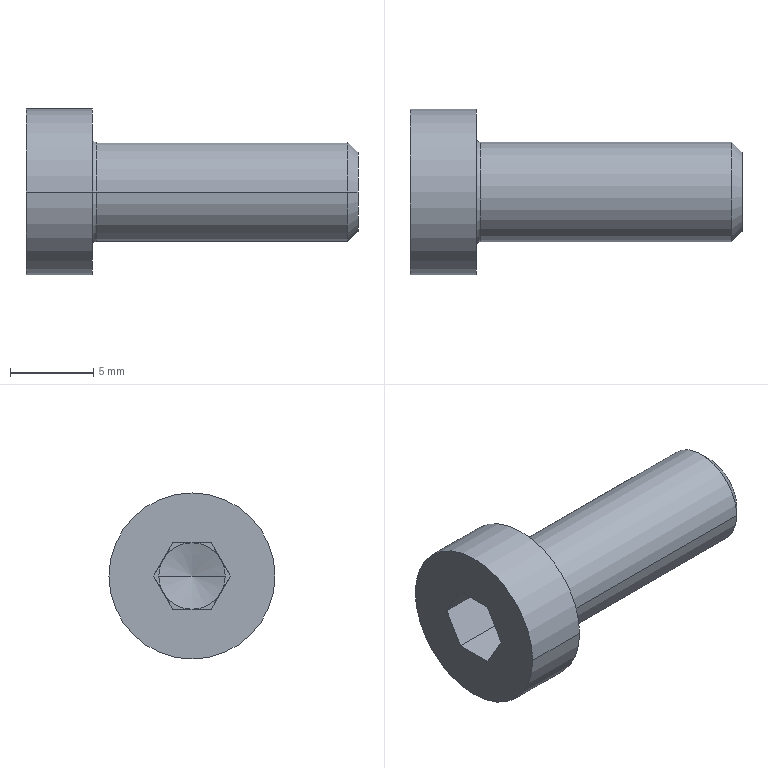Part | STEP file | CBSSTH6-16 | 1 solid | 25 faces | box 20 x 10 x 10 mm | volume 719.687 mm3 | plane 15 | cone 4 | cylinder 4 | torus 2 | commonest cylinder face diameters 6 x2 10 x2
STEP:
#1=CARTESIAN_POINT('',(-0.4641,0.,0.));
#2=VERTEX_POINT('',#1);
#3=CARTESIAN_POINT('',(-1.,-2.,0.));
#4=VERTEX_POINT('',#3);
#5=CARTESIAN_POINT('',(-0.4641,0.,0.));
#6=DIRECTION('',(-0.2588,-0.9659,0.));
#7=VECTOR('',#6,1000.);
#8=LINE('',#5,#7);
#9=EDGE_CURVE('',#2,#4,#8,.T.);
#10=ORIENTED_EDGE('',*,*,#9,.F.);
#11=CARTESIAN_POINT('',(-1.,2.,0.));
#12=VERTEX_POINT('',#11);
#13=CARTESIAN_POINT('',(-0.4641,0.,0.));
#14=DIRECTION('',(-0.2588,0.9659,0.));
#15=VECTOR('',#14,1000.);
#16=LINE('',#13,#15);
#17=EDGE_CURVE('',#2,#12,#16,.T.);
#18=ORIENTED_EDGE('',*,*,#17,.T.);
#19=CARTESIAN_POINT('',(-1.,1.732,-1.));
#20=VERTEX_POINT('',#19);
#21=CARTESIAN_POINT('',(-1.,0.,0.));
#22=DIRECTION('',(1.,0.,0.));
#23=DIRECTION('',(0.,1.,0.));
#24=AXIS2_PLACEMENT_3D('',#21,#22,#23);
#25=CIRCLE('',#24,2.);
#26=EDGE_CURVE('',#20,#12,#25,.T.);
#27=ORIENTED_EDGE('',*,*,#26,.F.);
#28=CARTESIAN_POINT('',(-1.,0.,-2.));
#29=VERTEX_POINT('',#28);
#30=CARTESIAN_POINT('',(-1.,0.,0.));
#31=DIRECTION('',(1.,0.,0.));
#32=DIRECTION('',(0.,1.,0.));
#33=AXIS2_PLACEMENT_3D('',#30,#31,#32);
#34=CIRCLE('',#33,2.);
#35=EDGE_CURVE('',#29,#20,#34,.T.);
#36=ORIENTED_EDGE('',*,*,#35,.F.);
#37=CARTESIAN_POINT('',(-1.,-1.732,-1.));
#38=VERTEX_POINT('',#37);
#39=CARTESIAN_POINT('',(-1.,0.,0.));
#40=DIRECTION('',(1.,0.,0.));
#41=DIRECTION('',(0.,1.,0.));
#42=AXIS2_PLACEMENT_3D('',#39,#40,#41);
#43=CIRCLE('',#42,2.);
#44=EDGE_CURVE('',#38,#29,#43,.T.);
#45=ORIENTED_EDGE('',*,*,#44,.F.);
#46=CARTESIAN_POINT('',(-1.,0.,0.));
#47=DIRECTION('',(1.,0.,0.));
#48=DIRECTION('',(0.,1.,0.));
#49=AXIS2_PLACEMENT_3D('',#46,#47,#48);
#50=CIRCLE('',#49,2.);
#51=EDGE_CURVE('',#4,#38,#50,.T.);
#52=ORIENTED_EDGE('',*,*,#51,.F.);
#53=EDGE_LOOP('',(#10,#18,#27,#36,#45,#52));
#54=FACE_OUTER_BOUND('',#53,.T.);
#55=CARTESIAN_POINT('',(-1000.464,0.,0.));
#56=DIRECTION('',(-1.,0.,0.));
#57=DIRECTION('',(0.,-1.,0.));
#58=AXIS2_PLACEMENT_3D('',#55,#56,#57);
#59=CONICAL_SURFACE('',#58,3732.051,1.309);
#60=ADVANCED_FACE('',(#54),#59,.F.);
#61=CARTESIAN_POINT('',(16.,2.387,0.));
#62=VERTEX_POINT('',#61);
#63=CARTESIAN_POINT('',(16.,-2.387,0.));
#64=VERTEX_POINT('',#63);
#65=CARTESIAN_POINT('',(16.,0.,0.));
#66=DIRECTION('',(1.,0.,0.));
#67=DIRECTION('',(0.,1.,0.));
#68=AXIS2_PLACEMENT_3D('',#65,#66,#67);
#69=CIRCLE('',#68,2.387);
#70=EDGE_CURVE('',#62,#64,#69,.T.);
#71=ORIENTED_EDGE('',*,*,#70,.F.);
#72=CARTESIAN_POINT('',(15.386,3.,0.));
#73=VERTEX_POINT('',#72);
#74=CARTESIAN_POINT('',(15.386,3.,0.));
#75=DIRECTION('',(-0.7071,0.7071,0.));
#76=VECTOR('',#75,1000.);
#77=LINE('',#74,#76);
#78=EDGE_CURVE('',#62,#73,#77,.T.);
#79=ORIENTED_EDGE('',*,*,#78,.T.);
#80=CARTESIAN_POINT('',(15.386,-3.,0.));
#81=VERTEX_POINT('',#80);
#82=CARTESIAN_POINT('',(15.386,0.,0.));
#83=DIRECTION('',(1.,0.,0.));
#84=DIRECTION('',(0.,1.,0.));
#85=AXIS2_PLACEMENT_3D('',#82,#83,#84);
#86=CIRCLE('',#85,3.);
#87=EDGE_CURVE('',#73,#81,#86,.T.);
#88=ORIENTED_EDGE('',*,*,#87,.T.);
#89=CARTESIAN_POINT('',(15.386,-3.,0.));
#90=DIRECTION('',(-0.7071,-0.7071,0.));
#91=VECTOR('',#90,1000.);
#92=LINE('',#89,#91);
#93=EDGE_CURVE('',#64,#81,#92,.T.);
#94=ORIENTED_EDGE('',*,*,#93,.F.);
#95=EDGE_LOOP('',(#71,#79,#88,#94));
#96=FACE_OUTER_BOUND('',#95,.T.);
#97=CARTESIAN_POINT('',(15.386,0.,0.));
#98=DIRECTION('',(-1.,0.,0.));
#99=DIRECTION('',(0.,-1.,0.));
#100=AXIS2_PLACEMENT_3D('',#97,#98,#99);
#101=CONICAL_SURFACE('',#100,3.,0.7854);
#102=ADVANCED_FACE('',(#96),#101,.T.);
#103=CARTESIAN_POINT('',(0.25,3.,0.));
#104=VERTEX_POINT('',#103);
#105=CARTESIAN_POINT('',(0.25,-3.,0.));
#106=VERTEX_POINT('',#105);
#107=CARTESIAN_POINT('',(0.25,0.,0.));
#108=DIRECTION('',(1.,0.,0.));
#109=DIRECTION('',(0.,1.,0.));
#110=AXIS2_PLACEMENT_3D('',#107,#108,#109);
#111=CIRCLE('',#110,3.);
#112=EDGE_CURVE('',#104,#106,#111,.T.);
#113=ORIENTED_EDGE('',*,*,#112,.T.);
#114=CARTESIAN_POINT('',(16.,-3.,0.));
#115=DIRECTION('',(1.,0.,0.));
#116=VECTOR('',#115,1000.);
#117=LINE('',#114,#116);
#118=EDGE_CURVE('',#106,#81,#117,.T.);
#119=ORIENTED_EDGE('',*,*,#118,.T.);
#120=ORIENTED_EDGE('',*,*,#87,.F.);
#121=CARTESIAN_POINT('',(16.,3.,0.));
#122=DIRECTION('',(1.,0.,0.));
#123=VECTOR('',#122,1000.);
#124=LINE('',#121,#123);
#125=EDGE_CURVE('',#104,#73,#124,.T.);
#126=ORIENTED_EDGE('',*,*,#125,.F.);
#127=EDGE_LOOP('',(#113,#119,#120,#126));
#128=FACE_OUTER_BOUND('',#127,.T.);
#129=CARTESIAN_POINT('',(16.,0.,0.));
#130=DIRECTION('',(1.,0.,0.));
#131=DIRECTION('',(0.,1.,0.));
#132=AXIS2_PLACEMENT_3D('',#129,#130,#131);
#133=CYLINDRICAL_SURFACE('',#132,3.);
#134=ADVANCED_FACE('',(#128),#133,.T.);
#135=CARTESIAN_POINT('',(0.25,0.,0.));
#136=DIRECTION('',(1.,0.,0.));
#137=DIRECTION('',(0.,1.,0.));
#138=AXIS2_PLACEMENT_3D('',#135,#136,#137);
#139=CIRCLE('',#138,3.);
#140=EDGE_CURVE('',#106,#104,#139,.T.);
#141=ORIENTED_EDGE('',*,*,#140,.F.);
#142=CARTESIAN_POINT('',(0.,-3.25,0.));
#143=VERTEX_POINT('',#142);
#144=CARTESIAN_POINT('',(0.25,-3.25,0.));
#145=DIRECTION('',(0.,0.,1.));
#146=DIRECTION('',(0.,-1.,0.));
#147=AXIS2_PLACEMENT_3D('',#144,#145,#146);
#148=CIRCLE('',#147,0.25);
#149=EDGE_CURVE('',#106,#143,#148,.T.);
#150=ORIENTED_EDGE('',*,*,#149,.T.);
#151=CARTESIAN_POINT('',(0.,3.25,0.));
#152=VERTEX_POINT('',#151);
#153=CARTESIAN_POINT('',(0.,0.,0.));
#154=DIRECTION('',(1.,0.,0.));
#155=DIRECTION('',(0.,1.,0.));
#156=AXIS2_PLACEMENT_3D('',#153,#154,#155);
#157=CIRCLE('',#156,3.25);
#158=EDGE_CURVE('',#143,#152,#157,.T.);
#159=ORIENTED_EDGE('',*,*,#158,.T.);
#160=CARTESIAN_POINT('',(0.25,3.25,0.));
#161=DIRECTION('',(0.,0.,-1.));
#162=DIRECTION('',(-1.,0.,0.));
#163=AXIS2_PLACEMENT_3D('',#160,#161,#162);
#164=CIRCLE('',#163,0.25);
#165=EDGE_CURVE('',#104,#152,#164,.T.);
#166=ORIENTED_EDGE('',*,*,#165,.F.);
#167=EDGE_LOOP('',(#141,#150,#159,#166));
#168=FACE_OUTER_BOUND('',#167,.T.);
#169=CARTESIAN_POINT('',(0.25,0.,0.));
#170=DIRECTION('',(1.,0.,0.));
#171=DIRECTION('',(0.,1.,0.));
#172=AXIS2_PLACEMENT_3D('',#169,#170,#171);
#173=TOROIDAL_SURFACE('',#172,3.25,0.25);
#174=ADVANCED_FACE('',(#168),#173,.F.);
#175=CARTESIAN_POINT('',(-4.,5.,0.));
#176=VERTEX_POINT('',#175);
#177=CARTESIAN_POINT('',(-4.,-5.,0.));
#178=VERTEX_POINT('',#177);
#179=CARTESIAN_POINT('',(-4.,0.,0.));
#180=DIRECTION('',(1.,0.,0.));
#181=DIRECTION('',(0.,1.,0.));
#182=AXIS2_PLACEMENT_3D('',#179,#180,#181);
#183=CIRCLE('',#182,5.);
#184=EDGE_CURVE('',#176,#178,#183,.T.);
#185=ORIENTED_EDGE('',*,*,#184,.T.);
#186=CARTESIAN_POINT('',(0.,-5.,0.));
#187=VERTEX_POINT('',#186);
#188=CARTESIAN_POINT('',(16.,-5.,0.));
#189=DIRECTION('',(1.,0.,0.));
#190=VECTOR('',#189,1000.);
#191=LINE('',#188,#190);
#192=EDGE_CURVE('',#178,#187,#191,.T.);
#193=ORIENTED_EDGE('',*,*,#192,.T.);
#194=CARTESIAN_POINT('',(0.,5.,0.));
#195=VERTEX_POINT('',#194);
#196=CARTESIAN_POINT('',(0.,0.,0.));
#197=DIRECTION('',(1.,0.,0.));
#198=DIRECTION('',(0.,1.,0.));
#199=AXIS2_PLACEMENT_3D('',#196,#197,#198);
#200=CIRCLE('',#199,5.);
#201=EDGE_CURVE('',#195,#187,#200,.T.);
#202=ORIENTED_EDGE('',*,*,#201,.F.);
#203=CARTESIAN_POINT('',(16.,5.,0.));
#204=DIRECTION('',(1.,0.,0.));
#205=VECTOR('',#204,1000.);
#206=LINE('',#203,#205);
#207=EDGE_CURVE('',#176,#195,#206,.T.);
#208=ORIENTED_EDGE('',*,*,#207,.F.);
#209=EDGE_LOOP('',(#185,#193,#202,#208));
#210=FACE_OUTER_BOUND('',#209,.T.);
#211=CARTESIAN_POINT('',(16.,0.,0.));
#212=DIRECTION('',(1.,0.,0.));
#213=DIRECTION('',(0.,1.,0.));
#214=AXIS2_PLACEMENT_3D('',#211,#212,#213);
#215=CYLINDRICAL_SURFACE('',#214,5.);
#216=ADVANCED_FACE('',(#210),#215,.T.);
#217=ORIENTED_EDGE('',*,*,#184,.F.);
#218=CARTESIAN_POINT('',(-4.,0.,0.));
#219=DIRECTION('',(1.,0.,0.));
#220=DIRECTION('',(0.,1.,0.));
#221=AXIS2_PLACEMENT_3D('',#218,#219,#220);
#222=CIRCLE('',#221,5.);
#223=EDGE_CURVE('',#178,#176,#222,.T.);
#224=ORIENTED_EDGE('',*,*,#223,.F.);
#225=EDGE_LOOP('',(#217,#224));
#226=FACE_OUTER_BOUND('',#225,.T.);
#227=CARTESIAN_POINT('',(-4.,-1.155,-2.));
#228=VERTEX_POINT('',#227);
#229=CARTESIAN_POINT('',(-4.,-2.309,0.));
#230=VERTEX_POINT('',#229);
#231=CARTESIAN_POINT('',(-4.,-1.232,-1.866));
#232=DIRECTION('',(0.,-0.5,0.866));
#233=VECTOR('',#232,1000.);
#234=LINE('',#231,#233);
#235=EDGE_CURVE('',#228,#230,#234,.T.);
#236=ORIENTED_EDGE('',*,*,#235,.F.);
#237=CARTESIAN_POINT('',(-4.,1.155,-2.));
#238=VERTEX_POINT('',#237);
#239=CARTESIAN_POINT('',(-4.,2.,-2.));
#240=DIRECTION('',(0.,-1.,0.));
#241=VECTOR('',#240,1000.);
#242=LINE('',#239,#241);
#243=EDGE_CURVE('',#238,#228,#242,.T.);
#244=ORIENTED_EDGE('',*,*,#243,.F.);
#245=CARTESIAN_POINT('',(-4.,2.309,0.));
#246=VERTEX_POINT('',#245);
#247=CARTESIAN_POINT('',(-4.,2.232,-0.134));
#248=DIRECTION('',(0.,-0.5,-0.866));
#249=VECTOR('',#248,1000.);
#250=LINE('',#247,#249);
#251=EDGE_CURVE('',#246,#238,#250,.T.);
#252=ORIENTED_EDGE('',*,*,#251,.F.);
#253=CARTESIAN_POINT('',(-4.,1.155,2.));
#254=VERTEX_POINT('',#253);
#255=CARTESIAN_POINT('',(-4.,2.232,0.134));
#256=DIRECTION('',(0.,0.5,-0.866));
#257=VECTOR('',#256,1000.);
#258=LINE('',#255,#257);
#259=EDGE_CURVE('',#254,#246,#258,.T.);
#260=ORIENTED_EDGE('',*,*,#259,.F.);
#261=CARTESIAN_POINT('',(-4.,-1.155,2.));
#262=VERTEX_POINT('',#261);
#263=CARTESIAN_POINT('',(-4.,2.,2.));
#264=DIRECTION('',(0.,1.,0.));
#265=VECTOR('',#264,1000.);
#266=LINE('',#263,#265);
#267=EDGE_CURVE('',#262,#254,#266,.T.);
#268=ORIENTED_EDGE('',*,*,#267,.F.);
#269=CARTESIAN_POINT('',(-4.,-1.232,1.866));
#270=DIRECTION('',(0.,0.5,0.866));
#271=VECTOR('',#270,1000.);
#272=LINE('',#269,#271);
#273=EDGE_CURVE('',#230,#262,#272,.T.);
#274=ORIENTED_EDGE('',*,*,#273,.F.);
#275=EDGE_LOOP('',(#236,#244,#252,#260,#268,#274));
#276=FACE_BOUND('',#275,.T.);
#277=CARTESIAN_POINT('',(-4.,2.,0.));
#278=DIRECTION('',(1.,0.,0.));
#279=DIRECTION('',(0.,1.,0.));
#280=AXIS2_PLACEMENT_3D('',#277,#278,#279);
#281=PLANE('',#280);
#282=ADVANCED_FACE('',(#226,#276),#281,.F.);
#283=ORIENTED_EDGE('',*,*,#192,.F.);
#284=ORIENTED_EDGE('',*,*,#223,.T.);
#285=ORIENTED_EDGE('',*,*,#207,.T.);
#286=CARTESIAN_POINT('',(0.,0.,0.));
#287=DIRECTION('',(1.,0.,0.));
#288=DIRECTION('',(0.,1.,0.));
#289=AXIS2_PLACEMENT_3D('',#286,#287,#288);
#290=CIRCLE('',#289,5.);
#291=EDGE_CURVE('',#187,#195,#290,.T.);
#292=ORIENTED_EDGE('',*,*,#291,.F.);
#293=EDGE_LOOP('',(#283,#284,#285,#292));
#294=FACE_OUTER_BOUND('',#293,.T.);
#295=CARTESIAN_POINT('',(16.,0.,0.));
#296=DIRECTION('',(1.,0.,0.));
#297=DIRECTION('',(0.,1.,0.));
#298=AXIS2_PLACEMENT_3D('',#295,#296,#297);
#299=CYLINDRICAL_SURFACE('',#298,5.);
#300=ADVANCED_FACE('',(#294),#299,.T.);
#301=CARTESIAN_POINT('',(0.,0.,0.));
#302=DIRECTION('',(1.,0.,0.));
#303=DIRECTION('',(0.,1.,0.));
#304=AXIS2_PLACEMENT_3D('',#301,#302,#303);
#305=CIRCLE('',#304,3.25);
#306=EDGE_CURVE('',#152,#143,#305,.T.);
#307=ORIENTED_EDGE('',*,*,#306,.F.);
#308=ORIENTED_EDGE('',*,*,#158,.F.);
#309=EDGE_LOOP('',(#307,#308));
#310=FACE_BOUND('',#309,.T.);
#311=ORIENTED_EDGE('',*,*,#201,.T.);
#312=ORIENTED_EDGE('',*,*,#291,.T.);
#313=EDGE_LOOP('',(#311,#312));
#314=FACE_OUTER_BOUND('',#313,.T.);
#315=CARTESIAN_POINT('',(0.,5.,0.));
#316=DIRECTION('',(-1.,0.,0.));
#317=DIRECTION('',(0.,-1.,0.));
#318=AXIS2_PLACEMENT_3D('',#315,#316,#317);
#319=PLANE('',#318);
#320=ADVANCED_FACE('',(#310,#314),#319,.F.);
#321=ORIENTED_EDGE('',*,*,#149,.F.);
#322=ORIENTED_EDGE('',*,*,#112,.F.);
#323=ORIENTED_EDGE('',*,*,#165,.T.);
#324=ORIENTED_EDGE('',*,*,#306,.T.);
#325=EDGE_LOOP('',(#321,#322,#323,#324));
#326=FACE_OUTER_BOUND('',#325,.T.);
#327=CARTESIAN_POINT('',(0.25,0.,0.));
#328=DIRECTION('',(1.,0.,0.));
#329=DIRECTION('',(0.,1.,0.));
#330=AXIS2_PLACEMENT_3D('',#327,#328,#329);
#331=TOROIDAL_SURFACE('',#330,3.25,0.25);
#332=ADVANCED_FACE('',(#326),#331,.F.);
#333=ORIENTED_EDGE('',*,*,#118,.F.);
#334=ORIENTED_EDGE('',*,*,#140,.T.);
#335=ORIENTED_EDGE('',*,*,#125,.T.);
#336=CARTESIAN_POINT('',(15.386,0.,0.));
#337=DIRECTION('',(1.,0.,0.));
#338=DIRECTION('',(0.,1.,0.));
#339=AXIS2_PLACEMENT_3D('',#336,#337,#338);
#340=CIRCLE('',#339,3.);
#341=EDGE_CURVE('',#81,#73,#340,.T.);
#342=ORIENTED_EDGE('',*,*,#341,.F.);
#343=EDGE_LOOP('',(#333,#334,#335,#342));
#344=FACE_OUTER_BOUND('',#343,.T.);
#345=CARTESIAN_POINT('',(16.,0.,0.));
#346=DIRECTION('',(1.,0.,0.));
#347=DIRECTION('',(0.,1.,0.));
#348=AXIS2_PLACEMENT_3D('',#345,#346,#347);
#349=CYLINDRICAL_SURFACE('',#348,3.);
#350=ADVANCED_FACE('',(#344),#349,.T.);
#351=ORIENTED_EDGE('',*,*,#78,.F.);
#352=CARTESIAN_POINT('',(16.,0.,0.));
#353=DIRECTION('',(1.,0.,0.));
#354=DIRECTION('',(0.,1.,0.));
#355=AXIS2_PLACEMENT_3D('',#352,#353,#354);
#356=CIRCLE('',#355,2.387);
#357=EDGE_CURVE('',#64,#62,#356,.T.);
#358=ORIENTED_EDGE('',*,*,#357,.F.);
#359=ORIENTED_EDGE('',*,*,#93,.T.);
#360=ORIENTED_EDGE('',*,*,#341,.T.);
#361=EDGE_LOOP('',(#351,#358,#359,#360));
#362=FACE_OUTER_BOUND('',#361,.T.);
#363=CARTESIAN_POINT('',(15.386,0.,0.));
#364=DIRECTION('',(-1.,0.,0.));
#365=DIRECTION('',(0.,-1.,0.));
#366=AXIS2_PLACEMENT_3D('',#363,#364,#365);
#367=CONICAL_SURFACE('',#366,3.,0.7854);
#368=ADVANCED_FACE('',(#362),#367,.T.);
#369=ORIENTED_EDGE('',*,*,#357,.T.);
#370=ORIENTED_EDGE('',*,*,#70,.T.);
#371=EDGE_LOOP('',(#369,#370));
#372=FACE_OUTER_BOUND('',#371,.T.);
#373=CARTESIAN_POINT('',(16.,2.387,0.));
#374=DIRECTION('',(-1.,0.,0.));
#375=DIRECTION('',(0.,-1.,0.));
#376=AXIS2_PLACEMENT_3D('',#373,#374,#375);
#377=PLANE('',#376);
#378=ADVANCED_FACE('',(#372),#377,.F.);
#379=CARTESIAN_POINT('',(-1.,-1.155,-2.));
#380=VERTEX_POINT('',#379);
#381=CARTESIAN_POINT('',(-1.,-1.155,-2.));
#382=DIRECTION('',(0.,1.,0.));
#383=VECTOR('',#382,1000.);
#384=LINE('',#381,#383);
#385=EDGE_CURVE('',#380,#29,#384,.T.);
#386=ORIENTED_EDGE('',*,*,#385,.F.);
#387=CARTESIAN_POINT('',(-1.,-2.309,0.));
#388=DIRECTION('',(0.,0.5,-0.866));
#389=VECTOR('',#388,1000.);
#390=LINE('',#387,#389);
#391=EDGE_CURVE('',#38,#380,#390,.T.);
#392=ORIENTED_EDGE('',*,*,#391,.F.);
#393=ORIENTED_EDGE('',*,*,#44,.T.);
#394=EDGE_LOOP('',(#386,#392,#393));
#395=FACE_OUTER_BOUND('',#394,.T.);
#396=CARTESIAN_POINT('',(-1.,0.,0.));
#397=DIRECTION('',(1.,0.,0.));
#398=DIRECTION('',(0.,0.,-1.));
#399=AXIS2_PLACEMENT_3D('',#396,#397,#398);
#400=PLANE('',#399);
#401=ADVANCED_FACE('',(#395),#400,.F.);
#402=CARTESIAN_POINT('',(-1.,-2.309,0.));
#403=VERTEX_POINT('',#402);
#404=CARTESIAN_POINT('',(-1.,-2.309,0.));
#405=DIRECTION('',(0.,0.5,-0.866));
#406=VECTOR('',#405,1000.);
#407=LINE('',#404,#406);
#408=EDGE_CURVE('',#403,#38,#407,.T.);
#409=ORIENTED_EDGE('',*,*,#408,.F.);
#410=CARTESIAN_POINT('',(-1.,-1.732,1.));
#411=VERTEX_POINT('',#410);
#412=CARTESIAN_POINT('',(-1.,-1.155,2.));
#413=DIRECTION('',(0.,-0.5,-0.866));
#414=VECTOR('',#413,1000.);
#415=LINE('',#412,#414);
#416=EDGE_CURVE('',#411,#403,#415,.T.);
#417=ORIENTED_EDGE('',*,*,#416,.F.);
#418=CARTESIAN_POINT('',(-1.,0.,0.));
#419=DIRECTION('',(1.,0.,0.));
#420=DIRECTION('',(0.,1.,0.));
#421=AXIS2_PLACEMENT_3D('',#418,#419,#420);
#422=CIRCLE('',#421,2.);
#423=EDGE_CURVE('',#411,#4,#422,.T.);
#424=ORIENTED_EDGE('',*,*,#423,.T.);
#425=ORIENTED_EDGE('',*,*,#51,.T.);
#426=EDGE_LOOP('',(#409,#417,#424,#425));
#427=FACE_OUTER_BOUND('',#426,.T.);
#428=CARTESIAN_POINT('',(-1.,0.,0.));
#429=DIRECTION('',(1.,0.,0.));
#430=DIRECTION('',(0.,0.,-1.));
#431=AXIS2_PLACEMENT_3D('',#428,#429,#430);
#432=PLANE('',#431);
#433=ADVANCED_FACE('',(#427),#432,.F.);
#434=CARTESIAN_POINT('',(-1.,-1.155,2.));
#435=VERTEX_POINT('',#434);
#436=CARTESIAN_POINT('',(-1.,-1.155,2.));
#437=DIRECTION('',(0.,-0.5,-0.866));
#438=VECTOR('',#437,1000.);
#439=LINE('',#436,#438);
#440=EDGE_CURVE('',#435,#411,#439,.T.);
#441=ORIENTED_EDGE('',*,*,#440,.F.);
#442=CARTESIAN_POINT('',(-1.,0.,2.));
#443=VERTEX_POINT('',#442);
#444=CARTESIAN_POINT('',(-1.,1.155,2.));
#445=DIRECTION('',(0.,-1.,0.));
#446=VECTOR('',#445,1000.);
#447=LINE('',#444,#446);
#448=EDGE_CURVE('',#443,#435,#447,.T.);
#449=ORIENTED_EDGE('',*,*,#448,.F.);
#450=CARTESIAN_POINT('',(-1.,0.,0.));
#451=DIRECTION('',(1.,0.,0.));
#452=DIRECTION('',(0.,1.,0.));
#453=AXIS2_PLACEMENT_3D('',#450,#451,#452);
#454=CIRCLE('',#453,2.);
#455=EDGE_CURVE('',#443,#411,#454,.T.);
#456=ORIENTED_EDGE('',*,*,#455,.T.);
#457=EDGE_LOOP('',(#441,#449,#456));
#458=FACE_OUTER_BOUND('',#457,.T.);
#459=CARTESIAN_POINT('',(-1.,0.,0.));
#460=DIRECTION('',(1.,0.,0.));
#461=DIRECTION('',(0.,0.,-1.));
#462=AXIS2_PLACEMENT_3D('',#459,#460,#461);
#463=PLANE('',#462);
#464=ADVANCED_FACE('',(#458),#463,.F.);
#465=CARTESIAN_POINT('',(-1.,1.155,2.));
#466=VERTEX_POINT('',#465);
#467=CARTESIAN_POINT('',(-1.,1.155,2.));
#468=DIRECTION('',(0.,-1.,0.));
#469=VECTOR('',#468,1000.);
#470=LINE('',#467,#469);
#471=EDGE_CURVE('',#466,#443,#470,.T.);
#472=ORIENTED_EDGE('',*,*,#471,.F.);
#473=CARTESIAN_POINT('',(-1.,1.732,1.));
#474=VERTEX_POINT('',#473);
#475=CARTESIAN_POINT('',(-1.,2.309,0.));
#476=DIRECTION('',(0.,-0.5,0.866));
#477=VECTOR('',#476,1000.);
#478=LINE('',#475,#477);
#479=EDGE_CURVE('',#474,#466,#478,.T.);
#480=ORIENTED_EDGE('',*,*,#479,.F.);
#481=CARTESIAN_POINT('',(-1.,0.,0.));
#482=DIRECTION('',(1.,0.,0.));
#483=DIRECTION('',(0.,1.,0.));
#484=AXIS2_PLACEMENT_3D('',#481,#482,#483);
#485=CIRCLE('',#484,2.);
#486=EDGE_CURVE('',#474,#443,#485,.T.);
#487=ORIENTED_EDGE('',*,*,#486,.T.);
#488=EDGE_LOOP('',(#472,#480,#487));
#489=FACE_OUTER_BOUND('',#488,.T.);
#490=CARTESIAN_POINT('',(-1.,0.,0.));
#491=DIRECTION('',(1.,0.,0.));
#492=DIRECTION('',(0.,0.,-1.));
#493=AXIS2_PLACEMENT_3D('',#490,#491,#492);
#494=PLANE('',#493);
#495=ADVANCED_FACE('',(#489),#494,.F.);
#496=CARTESIAN_POINT('',(-1.,2.309,0.));
#497=VERTEX_POINT('',#496);
#498=CARTESIAN_POINT('',(-1.,2.309,0.));
#499=DIRECTION('',(0.,-0.5,0.866));
#500=VECTOR('',#499,1000.);
#501=LINE('',#498,#500);
#502=EDGE_CURVE('',#497,#474,#501,.T.);
#503=ORIENTED_EDGE('',*,*,#502,.F.);
#504=CARTESIAN_POINT('',(-1.,1.155,-2.));
#505=DIRECTION('',(0.,0.5,0.866));
#506=VECTOR('',#505,1000.);
#507=LINE('',#504,#506);
#508=EDGE_CURVE('',#20,#497,#507,.T.);
#509=ORIENTED_EDGE('',*,*,#508,.F.);
#510=ORIENTED_EDGE('',*,*,#26,.T.);
#511=CARTESIAN_POINT('',(-1.,0.,0.));
#512=DIRECTION('',(1.,0.,0.));
#513=DIRECTION('',(0.,1.,0.));
#514=AXIS2_PLACEMENT_3D('',#511,#512,#513);
#515=CIRCLE('',#514,2.);
#516=EDGE_CURVE('',#12,#474,#515,.T.);
#517=ORIENTED_EDGE('',*,*,#516,.T.);
#518=EDGE_LOOP('',(#503,#509,#510,#517));
#519=FACE_OUTER_BOUND('',#518,.T.);
#520=CARTESIAN_POINT('',(-1.,0.,0.));
#521=DIRECTION('',(1.,0.,0.));
#522=DIRECTION('',(0.,0.,-1.));
#523=AXIS2_PLACEMENT_3D('',#520,#521,#522);
#524=PLANE('',#523);
#525=ADVANCED_FACE('',(#519),#524,.F.);
#526=CARTESIAN_POINT('',(-1.,1.155,-2.));
#527=VERTEX_POINT('',#526);
#528=CARTESIAN_POINT('',(-1.,1.155,-2.));
#529=DIRECTION('',(0.,0.5,0.866));
#530=VECTOR('',#529,1000.);
#531=LINE('',#528,#530);
#532=EDGE_CURVE('',#527,#20,#531,.T.);
#533=ORIENTED_EDGE('',*,*,#532,.F.);
#534=CARTESIAN_POINT('',(-1.,-1.155,-2.));
#535=DIRECTION('',(0.,1.,0.));
#536=VECTOR('',#535,1000.);
#537=LINE('',#534,#536);
#538=EDGE_CURVE('',#29,#527,#537,.T.);
#539=ORIENTED_EDGE('',*,*,#538,.F.);
#540=ORIENTED_EDGE('',*,*,#35,.T.);
#541=EDGE_LOOP('',(#533,#539,#540));
#542=FACE_OUTER_BOUND('',#541,.T.);
#543=CARTESIAN_POINT('',(-1.,0.,0.));
#544=DIRECTION('',(1.,0.,0.));
#545=DIRECTION('',(0.,0.,-1.));
#546=AXIS2_PLACEMENT_3D('',#543,#544,#545);
#547=PLANE('',#546);
#548=ADVANCED_FACE('',(#542),#547,.F.);
#549=ORIENTED_EDGE('',*,*,#471,.T.);
#550=ORIENTED_EDGE('',*,*,#448,.T.);
#551=CARTESIAN_POINT('',(-1.,-1.155,2.));
#552=DIRECTION('',(-1.,0.,0.));
#553=VECTOR('',#552,1000.);
#554=LINE('',#551,#553);
#555=EDGE_CURVE('',#435,#262,#554,.T.);
#556=ORIENTED_EDGE('',*,*,#555,.T.);
#557=ORIENTED_EDGE('',*,*,#267,.T.);
#558=CARTESIAN_POINT('',(-1.,1.155,2.));
#559=DIRECTION('',(-1.,0.,0.));
#560=VECTOR('',#559,1000.);
#561=LINE('',#558,#560);
#562=EDGE_CURVE('',#466,#254,#561,.T.);
#563=ORIENTED_EDGE('',*,*,#562,.F.);
#564=EDGE_LOOP('',(#549,#550,#556,#557,#563));
#565=FACE_OUTER_BOUND('',#564,.T.);
#566=CARTESIAN_POINT('',(-1.,1.155,2.));
#567=DIRECTION('',(0.,0.,-1.));
#568=DIRECTION('',(-1.,0.,0.));
#569=AXIS2_PLACEMENT_3D('',#566,#567,#568);
#570=PLANE('',#569);
#571=ADVANCED_FACE('',(#565),#570,.T.);
#572=ORIENTED_EDGE('',*,*,#440,.T.);
#573=ORIENTED_EDGE('',*,*,#416,.T.);
#574=CARTESIAN_POINT('',(-1.,-2.309,0.));
#575=DIRECTION('',(-1.,0.,0.));
#576=VECTOR('',#575,1000.);
#577=LINE('',#574,#576);
#578=EDGE_CURVE('',#403,#230,#577,.T.);
#579=ORIENTED_EDGE('',*,*,#578,.T.);
#580=ORIENTED_EDGE('',*,*,#273,.T.);
#581=ORIENTED_EDGE('',*,*,#555,.F.);
#582=EDGE_LOOP('',(#572,#573,#579,#580,#581));
#583=FACE_OUTER_BOUND('',#582,.T.);
#584=CARTESIAN_POINT('',(-1.,-1.155,2.));
#585=DIRECTION('',(0.,0.866,-0.5));
#586=DIRECTION('',(0.,0.5,0.866));
#587=AXIS2_PLACEMENT_3D('',#584,#585,#586);
#588=PLANE('',#587);
#589=ADVANCED_FACE('',(#583),#588,.T.);
#590=ORIENTED_EDGE('',*,*,#408,.T.);
#591=ORIENTED_EDGE('',*,*,#391,.T.);
#592=CARTESIAN_POINT('',(-1.,-1.155,-2.));
#593=DIRECTION('',(-1.,0.,0.));
#594=VECTOR('',#593,1000.);
#595=LINE('',#592,#594);
#596=EDGE_CURVE('',#380,#228,#595,.T.);
#597=ORIENTED_EDGE('',*,*,#596,.T.);
#598=ORIENTED_EDGE('',*,*,#235,.T.);
#599=ORIENTED_EDGE('',*,*,#578,.F.);
#600=EDGE_LOOP('',(#590,#591,#597,#598,#599));
#601=FACE_OUTER_BOUND('',#600,.T.);
#602=CARTESIAN_POINT('',(-1.,-2.309,0.));
#603=DIRECTION('',(0.,0.866,0.5));
#604=DIRECTION('',(0.,-0.5,0.866));
#605=AXIS2_PLACEMENT_3D('',#602,#603,#604);
#606=PLANE('',#605);
#607=ADVANCED_FACE('',(#601),#606,.T.);
#608=ORIENTED_EDGE('',*,*,#385,.T.);
#609=ORIENTED_EDGE('',*,*,#538,.T.);
#610=CARTESIAN_POINT('',(-1.,1.155,-2.));
#611=DIRECTION('',(-1.,0.,0.));
#612=VECTOR('',#611,1000.);
#613=LINE('',#610,#612);
#614=EDGE_CURVE('',#527,#238,#613,.T.);
#615=ORIENTED_EDGE('',*,*,#614,.T.);
#616=ORIENTED_EDGE('',*,*,#243,.T.);
#617=ORIENTED_EDGE('',*,*,#596,.F.);
#618=EDGE_LOOP('',(#608,#609,#615,#616,#617));
#619=FACE_OUTER_BOUND('',#618,.T.);
#620=CARTESIAN_POINT('',(-1.,-1.155,-2.));
#621=DIRECTION('',(0.,0.,1.));
#622=DIRECTION('',(1.,0.,0.));
#623=AXIS2_PLACEMENT_3D('',#620,#621,#622);
#624=PLANE('',#623);
#625=ADVANCED_FACE('',(#619),#624,.T.);
#626=ORIENTED_EDGE('',*,*,#532,.T.);
#627=ORIENTED_EDGE('',*,*,#508,.T.);
#628=CARTESIAN_POINT('',(-1.,2.309,0.));
#629=DIRECTION('',(-1.,0.,0.));
#630=VECTOR('',#629,1000.);
#631=LINE('',#628,#630);
#632=EDGE_CURVE('',#497,#246,#631,.T.);
#633=ORIENTED_EDGE('',*,*,#632,.T.);
#634=ORIENTED_EDGE('',*,*,#251,.T.);
#635=ORIENTED_EDGE('',*,*,#614,.F.);
#636=EDGE_LOOP('',(#626,#627,#633,#634,#635));
#637=FACE_OUTER_BOUND('',#636,.T.);
#638=CARTESIAN_POINT('',(-1.,1.155,-2.));
#639=DIRECTION('',(0.,-0.866,0.5));
#640=DIRECTION('',(0.,-0.5,-0.866));
#641=AXIS2_PLACEMENT_3D('',#638,#639,#640);
#642=PLANE('',#641);
#643=ADVANCED_FACE('',(#637),#642,.T.);
#644=ORIENTED_EDGE('',*,*,#502,.T.);
#645=ORIENTED_EDGE('',*,*,#479,.T.);
#646=ORIENTED_EDGE('',*,*,#562,.T.);
#647=ORIENTED_EDGE('',*,*,#259,.T.);
#648=ORIENTED_EDGE('',*,*,#632,.F.);
#649=EDGE_LOOP('',(#644,#645,#646,#647,#648));
#650=FACE_OUTER_BOUND('',#649,.T.);
#651=CARTESIAN_POINT('',(-1.,2.309,0.));
#652=DIRECTION('',(0.,-0.866,-0.5));
#653=DIRECTION('',(0.,0.5,-0.866));
#654=AXIS2_PLACEMENT_3D('',#651,#652,#653);
#655=PLANE('',#654);
#656=ADVANCED_FACE('',(#650),#655,.T.);
#657=ORIENTED_EDGE('',*,*,#17,.F.);
#658=ORIENTED_EDGE('',*,*,#9,.T.);
#659=ORIENTED_EDGE('',*,*,#423,.F.);
#660=ORIENTED_EDGE('',*,*,#455,.F.);
#661=ORIENTED_EDGE('',*,*,#486,.F.);
#662=ORIENTED_EDGE('',*,*,#516,.F.);
#663=EDGE_LOOP('',(#657,#658,#659,#660,#661,#662));
#664=FACE_OUTER_BOUND('',#663,.T.);
#665=CARTESIAN_POINT('',(-1000.464,0.,0.));
#666=DIRECTION('',(-1.,0.,0.));
#667=DIRECTION('',(0.,-1.,0.));
#668=AXIS2_PLACEMENT_3D('',#665,#666,#667);
#669=CONICAL_SURFACE('',#668,3732.051,1.309);
#670=ADVANCED_FACE('',(#664),#669,.F.);
#671=CLOSED_SHELL('',(#60,#102,#134,#174,#216,#282,#300,#320,#332,#350,#368,#378,#401,#433,#464,#495,#525,#548,#571,#589,#607,#625,#643,#656,#670));
#672=MANIFOLD_SOLID_BREP('',#671);
#673=CARTESIAN_POINT('',(0.,0.,0.));
#674=DIRECTION('',(0.,0.,1.));
#675=DIRECTION('',(1.,0.,0.));
#676=AXIS2_PLACEMENT_3D('',#673,#674,#675);
#677=(LENGTH_UNIT()NAMED_UNIT(*)SI_UNIT(.MILLI.,.METRE.));
#678=UNCERTAINTY_MEASURE_WITH_UNIT(LENGTH_MEASURE(0.00001),#677,'','');
#679=(NAMED_UNIT(*)PLANE_ANGLE_UNIT()SI_UNIT($,.RADIAN.));
#680=(NAMED_UNIT(*)SI_UNIT($,.STERADIAN.)SOLID_ANGLE_UNIT());
#681=(GEOMETRIC_REPRESENTATION_CONTEXT(3)GLOBAL_UNCERTAINTY_ASSIGNED_CONTEXT((#678))GLOBAL_UNIT_ASSIGNED_CONTEXT((#677,#679,#680))REPRESENTATION_CONTEXT('',''));
#682=ADVANCED_BREP_SHAPE_REPRESENTATION('',(#672,#676),#681);